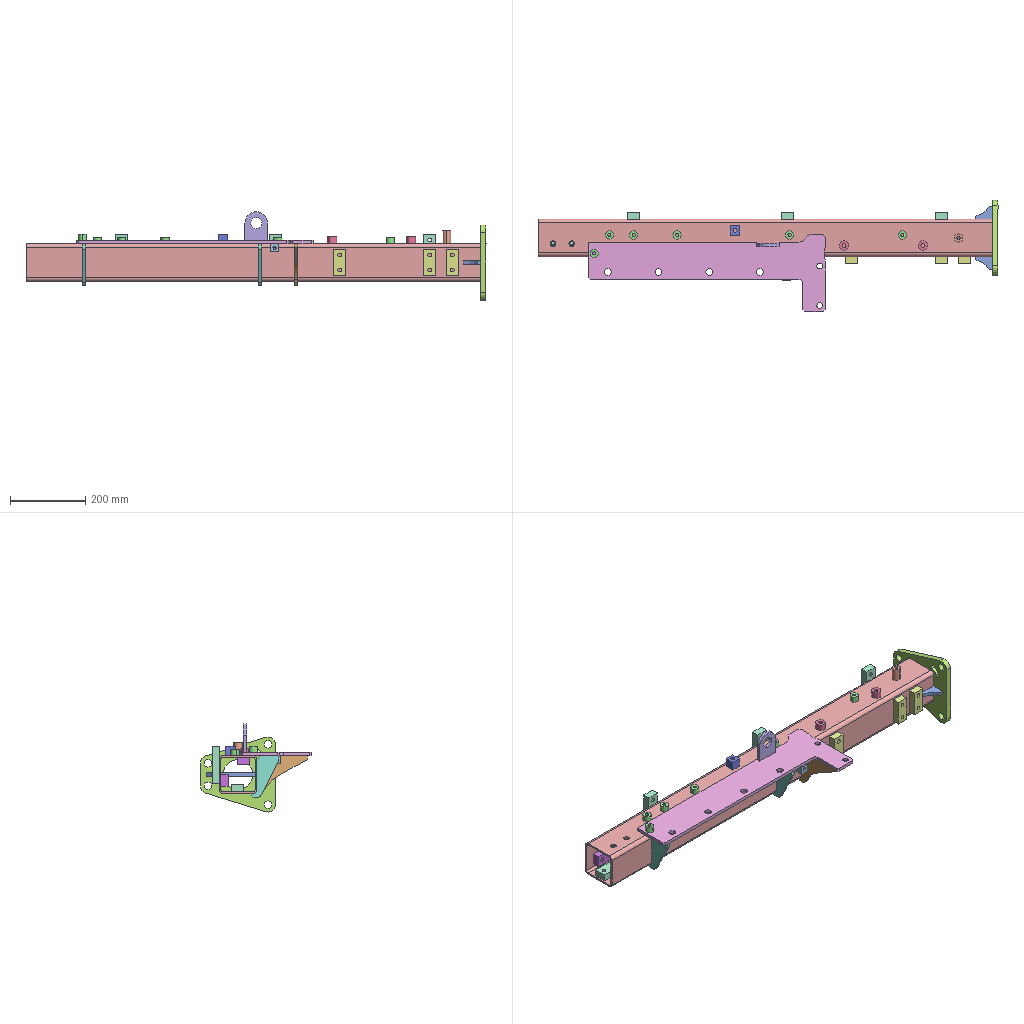Assembly | SolidWorks | 15 different items | 28 placed | box 1225 x 296 x 234 mm
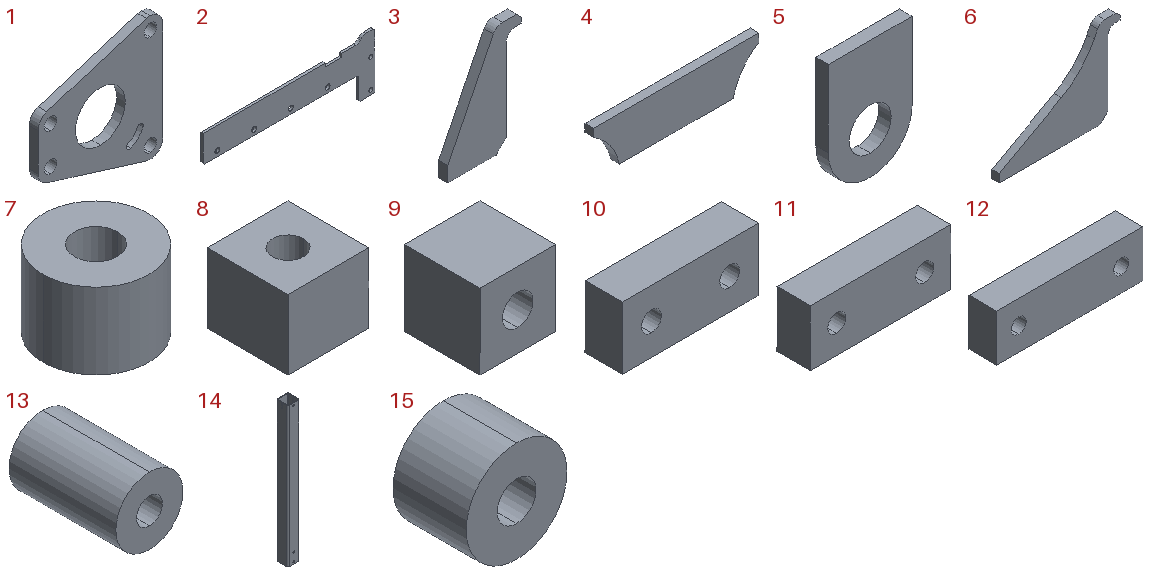Parts list (item | quantity | size | volume | features):
1 | x1 | 200 x 14 x 199.722 mm | 327210 mm3 | features FlatPattern 1, SMBaseFlange 1, SheetMetal 1
2 | x1 | 630 x 9 x 205 mm | 602554 mm3 | features FlatPattern 1, SMBaseFlange 1, SheetMetal 1
3 | x2 | 72.5 x 9 x 110 mm | 37505 mm3 | features FlatPattern 1, SMBaseFlange 1, SheetMetal 1
4 | x1 | 170 x 9 x 45 mm | 57559 mm3 | features FlatPattern 1, SMBaseFlange 1, SheetMetal 1
5 | x1 | 60 x 9 x 85 mm | 36062 mm3 | features FlatPattern 1, SMBaseFlange 1, SheetMetal 1
6 | x1 | 150 x 9 x 110 mm | 64944 mm3 | features FlatPattern 1, SMBaseFlange 1, SheetMetal 1
7 | x2 | 25 x 25 x 18 mm | 7365 mm3 | features Extrusion 1, HoleWzd 1
8 | x1 | 22 x 22 x 19 mm | 8118 mm3 | features 3DProfileFeature 1, Extrusion 1, HoleWzd 1
9 | x1 | 25 x 25 x 25 mm | 13582 mm3 | features Extrusion 1, HoleWzd 1
10 | x3 | 70 x 19 x 32 mm | 39455 mm3 | features FlatPattern 1, HoleWzd 1, SMBaseFlange 1, SheetMetal 1
11 | x2 | 80 x 19 x 32 mm | 45535 mm3 | features FlatPattern 1, HoleWzd 1, SMBaseFlange 1, SheetMetal 1
12 | x4 | 100 x 19 x 32 mm | 57695 mm3 | features FlatPattern 1, HoleWzd 1, SMBaseFlange 1, SheetMetal 1
13 | x1 | 22 x 35 x 22 mm | 11319 mm3 | features Extrusion 1, HoleWzd 1
14 | x1 | 100 x 100 x 1211 mm | 1999990 mm3 | features ICE 4, Attribute 1, Extrusion 1
15 | x6 | 22 x 16 x 22 mm | 5174 mm3 | features Extrusion 1, HoleWzd 1
Mates (type | each side: item.copy, entity, surface, feature):
Coincident | 14.1 face plane Cut-Extrude4 | 4.1 face plane Base-Flange1 | 2 times
DistanceDim | 4.1 face plane Base-Flange1 | 14.1 face plane Boss-Extrude1
Coincident | 14.1 face plane Boss-Extrude1 | 1.1 face plane Base-Flange1
DistanceDim | 1.1 face cylinder Base-Flange1 | 14.1 face plane Boss-Extrude1 | 2 times
Parallel | 14.1 face plane Boss-Extrude1 | 1.1 face plane Base-Flange1
Coincident | 14.1 face plane Boss-Extrude1 | 2.1 face plane Base-Flange1
DistanceDim | 2.1 face plane Base-Flange1 | 14.1 face plane Boss-Extrude1
DistanceDim | 2.1 face plane Base-Flange1 | 1.1 face plane Base-Flange1
Coincident | 14.1 face plane Boss-Extrude1 | 3.1 face plane Base-Flange1
Coincident | 2.1 face plane Base-Flange1 | 3.1 face plane Base-Flange1
DistanceDim | 2.1 face cylinder Base-Flange1 | 3.1 face plane Base-Flange1
Coincident | 14.1 face plane Boss-Extrude1 | 6.1 face plane Base-Flange1
Coincident | 2.1 face plane Base-Flange1 | 6.1 face plane Base-Flange1
DistanceDim | 3.1 face plane Base-Flange1 | 6.1 face plane Base-Flange1
Coincident | 14.1 face plane Boss-Extrude1 | 5.1 face plane Base-Flange1
Coincident | 2.1 face plane Base-Flange1 | 5.1 face plane Base-Flange1 | 2 times
Coincident | 14.1 face plane Boss-Extrude1 | 15.1 face plane Boss-Extrude1
DistanceDim | 15.1 face cylinder Boss-Extrude1 | 1.1 face plane Base-Flange1
DistanceDim | 14.1 face plane Boss-Extrude1 | 15.1 face cylinder Boss-Extrude1
Coincident | 14.1 face plane Boss-Extrude1 | 15.2 face plane Boss-Extrude1
DistanceDim | 14.1 face plane Boss-Extrude1 | 15.2 face cylinder Boss-Extrude1
DistanceDim | 15.3 face cylinder Boss-Extrude1 | 15.2 face cylinder Boss-Extrude1
Coincident | 14.1 face plane Boss-Extrude1 | 15.4 face plane Boss-Extrude1
DistanceDim | 14.1 face plane Boss-Extrude1 | 15.4 face cylinder Boss-Extrude1
DistanceDim | 15.2 face cylinder Boss-Extrude1 | 15.4 face cylinder Boss-Extrude1
Coincident | 2.1 face plane Base-Flange1 | 15.5 face plane Boss-Extrude1
DistanceDim | 14.1 face plane Boss-Extrude1 | 15.5 face cylinder Boss-Extrude1
DistanceDim | 15.5 face cylinder Boss-Extrude1 | 1.1 face plane Base-Flange1
Coincident | 14.1 face plane Boss-Extrude1 | 7.1 face plane Boss-Extrude1
DistanceDim | 14.1 face plane Boss-Extrude1 | 7.1 face cylinder Boss-Extrude1
DistanceDim | 7.1 face cylinder Boss-Extrude1 | 1.1 face plane Base-Flange1
Coincident | 2.1 face plane Base-Flange1 | 8.1 face plane Boss-Extrude1
DistanceDim | 2.1 face plane Base-Flange1 | 8.1 face plane Boss-Extrude1
DistanceDim | 8.1 face plane Boss-Extrude1 | 2.1 face plane Base-Flange1
Coincident | 14.1 face plane Boss-Extrude1 | 10.1 face plane Base-Flange1
DistanceDim | 10.1 face plane Base-Flange1 | 1.1 face plane Base-Flange1
DistanceDim | 14.1 face plane Boss-Extrude1 | 10.1 face plane Base-Flange1
Coincident | 14.1 face plane Boss-Extrude1 | 10.2 face plane Base-Flange1
Coincident | 10.1 face plane Base-Flange1 | 10.2 face plane Base-Flange1
DistanceDim | 10.1 face plane Base-Flange1 | 10.2 face plane Base-Flange1
Coincident | 14.1 face plane Boss-Extrude1 | 10.3 face plane Base-Flange1
Coincident | 10.2 face plane Base-Flange1 | 10.3 face plane Base-Flange1
DistanceDim | 10.1 face plane Base-Flange1 | 10.3 face plane Base-Flange1
Coincident | 14.1 face plane Boss-Extrude1 | 11.1 face plane Base-Flange1
Concentric | 14.1 face cylinder Cut-Extrude3 | 11.1 face cylinder M12 Tapped Hole1 | 2 times
Coincident | 14.1 face plane Boss-Extrude1 | 11.2 face plane Base-Flange1
Concentric | 14.1 face cylinder Cut-Extrude1 | 11.2 face cylinder M12 Tapped Hole1 | 2 times
Coincident | 14.1 face plane Boss-Extrude1 | 12.1 face plane Base-Flange1
Concentric | 14.1 face cylinder Cut-Extrude2 | 12.1 face cylinder M12 Tapped Hole1 | 2 times
Coincident | 14.1 face plane Boss-Extrude1 | 12.2 face plane Base-Flange1
DistanceDim | 1.1 face plane Base-Flange1 | 12.2 face plane Base-Flange1
DistanceDim | 14.1 face plane Boss-Extrude1 | 12.2 face cylinder M12 Tapped Hole1
Coincident | 14.1 face plane Boss-Extrude1 | 13.1 face plane Boss-Extrude1
DistanceDim | 14.1 face plane Boss-Extrude1 | 13.1 face cylinder Boss-Extrude1
DistanceDim | 13.1 face cylinder Boss-Extrude1 | 1.1 face plane Base-Flange1
Coincident | 14.1 face plane Boss-Extrude1 | 9.1 face plane Boss-Extrude1
DistanceDim | 1.1 face plane Base-Flange1 | 9.1 face plane Boss-Extrude1
DistanceDim | 14.1 face plane Boss-Extrude1 | 9.1 face plane Boss-Extrude1